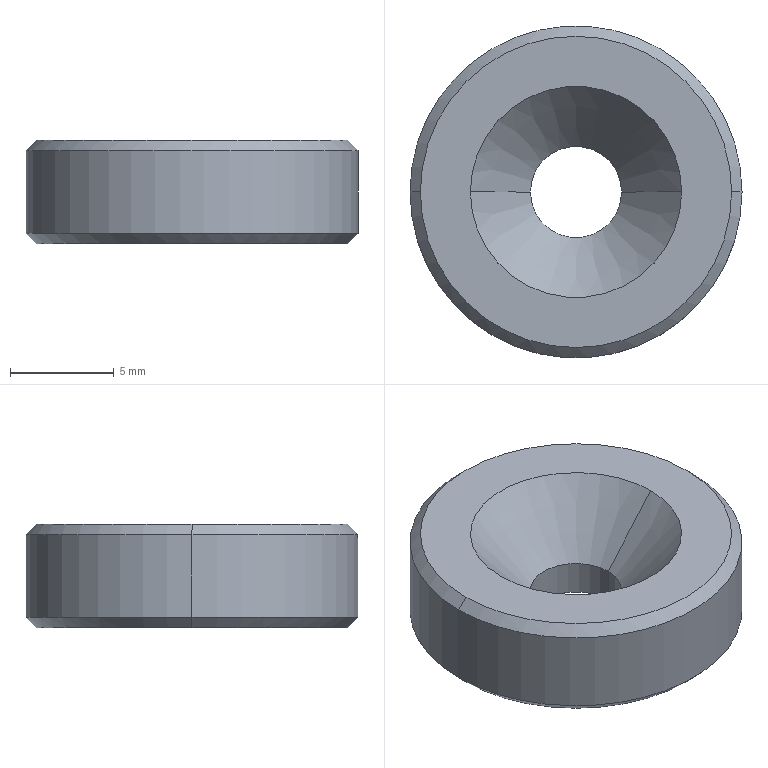Part | STEP file | 4-20.sldasm-Part-275 | 1 solid | 12 faces | box 16 x 16 x 5 mm | volume 821.609 mm3 | cone 6 | cylinder 4 | plane 2 | commonest cylinder face diameters 4.4 x2 16 x2
STEP:
#1=CARTESIAN_POINT('',(85.5,0.,-135.));
#2=VERTEX_POINT('',#1);
#3=CARTESIAN_POINT('',(100.5,0.,-135.));
#4=VERTEX_POINT('',#3);
#5=CARTESIAN_POINT('',(93.,0.,-135.));
#6=DIRECTION('',(0.,0.,1.));
#7=DIRECTION('',(-1.,0.,0.));
#8=AXIS2_PLACEMENT_3D('',#5,#6,#7);
#9=CIRCLE('',#8,7.5);
#10=EDGE_CURVE('',#2,#4,#9,.T.);
#11=ORIENTED_EDGE('',*,*,#10,.F.);
#12=CARTESIAN_POINT('',(85.,0.,-135.5));
#13=VERTEX_POINT('',#12);
#14=CARTESIAN_POINT('',(85.,0.,-135.5));
#15=DIRECTION('',(-0.7071,0.,-0.7071));
#16=VECTOR('',#15,1000.);
#17=LINE('',#14,#16);
#18=EDGE_CURVE('',#2,#13,#17,.T.);
#19=ORIENTED_EDGE('',*,*,#18,.T.);
#20=CARTESIAN_POINT('',(101.,0.,-135.5));
#21=VERTEX_POINT('',#20);
#22=CARTESIAN_POINT('',(93.,0.,-135.5));
#23=DIRECTION('',(0.,0.,-1.));
#24=DIRECTION('',(-1.,0.,0.));
#25=AXIS2_PLACEMENT_3D('',#22,#23,#24);
#26=CIRCLE('',#25,8.);
#27=EDGE_CURVE('',#21,#13,#26,.T.);
#28=ORIENTED_EDGE('',*,*,#27,.F.);
#29=CARTESIAN_POINT('',(101.,0.,-135.5));
#30=DIRECTION('',(0.7071,0.,-0.7071));
#31=VECTOR('',#30,1000.);
#32=LINE('',#29,#31);
#33=EDGE_CURVE('',#4,#21,#32,.T.);
#34=ORIENTED_EDGE('',*,*,#33,.F.);
#35=EDGE_LOOP('',(#11,#19,#28,#34));
#36=FACE_OUTER_BOUND('',#35,.T.);
#37=CARTESIAN_POINT('',(93.,0.,-135.5));
#38=DIRECTION('',(0.,0.,-1.));
#39=DIRECTION('',(1.,0.,0.));
#40=AXIS2_PLACEMENT_3D('',#37,#38,#39);
#41=CONICAL_SURFACE('',#40,8.,0.7854);
#42=ADVANCED_FACE('',(#36),#41,.T.);
#43=CARTESIAN_POINT('',(100.5,0.,-140.));
#44=VERTEX_POINT('',#43);
#45=CARTESIAN_POINT('',(85.5,0.,-140.));
#46=VERTEX_POINT('',#45);
#47=CARTESIAN_POINT('',(93.,0.,-140.));
#48=DIRECTION('',(0.,0.,-1.));
#49=DIRECTION('',(1.,0.,0.));
#50=AXIS2_PLACEMENT_3D('',#47,#48,#49);
#51=CIRCLE('',#50,7.5);
#52=EDGE_CURVE('',#44,#46,#51,.T.);
#53=ORIENTED_EDGE('',*,*,#52,.F.);
#54=CARTESIAN_POINT('',(101.,0.,-139.5));
#55=VERTEX_POINT('',#54);
#56=CARTESIAN_POINT('',(101.,0.,-139.5));
#57=DIRECTION('',(0.7071,0.,0.7071));
#58=VECTOR('',#57,1000.);
#59=LINE('',#56,#58);
#60=EDGE_CURVE('',#44,#55,#59,.T.);
#61=ORIENTED_EDGE('',*,*,#60,.T.);
#62=CARTESIAN_POINT('',(85.,0.,-139.5));
#63=VERTEX_POINT('',#62);
#64=CARTESIAN_POINT('',(93.,0.,-139.5));
#65=DIRECTION('',(0.,0.,1.));
#66=DIRECTION('',(1.,0.,0.));
#67=AXIS2_PLACEMENT_3D('',#64,#65,#66);
#68=CIRCLE('',#67,8.);
#69=EDGE_CURVE('',#63,#55,#68,.T.);
#70=ORIENTED_EDGE('',*,*,#69,.F.);
#71=CARTESIAN_POINT('',(85.,0.,-139.5));
#72=DIRECTION('',(-0.7071,0.,0.7071));
#73=VECTOR('',#72,1000.);
#74=LINE('',#71,#73);
#75=EDGE_CURVE('',#46,#63,#74,.T.);
#76=ORIENTED_EDGE('',*,*,#75,.F.);
#77=EDGE_LOOP('',(#53,#61,#70,#76));
#78=FACE_OUTER_BOUND('',#77,.T.);
#79=CARTESIAN_POINT('',(93.,0.,-139.5));
#80=DIRECTION('',(0.,0.,1.));
#81=DIRECTION('',(-1.,0.,0.));
#82=AXIS2_PLACEMENT_3D('',#79,#80,#81);
#83=CONICAL_SURFACE('',#82,8.,0.7854);
#84=ADVANCED_FACE('',(#78),#83,.T.);
#85=CARTESIAN_POINT('',(95.2,0.,-138.323));
#86=VERTEX_POINT('',#85);
#87=CARTESIAN_POINT('',(90.8,0.,-138.323));
#88=VERTEX_POINT('',#87);
#89=CARTESIAN_POINT('',(93.,0.,-138.323));
#90=DIRECTION('',(0.,0.,1.));
#91=DIRECTION('',(-1.,0.,0.));
#92=AXIS2_PLACEMENT_3D('',#89,#90,#91);
#93=CIRCLE('',#92,2.2);
#94=EDGE_CURVE('',#86,#88,#93,.T.);
#95=ORIENTED_EDGE('',*,*,#94,.F.);
#96=CARTESIAN_POINT('',(98.089,0.,-135.));
#97=VERTEX_POINT('',#96);
#98=CARTESIAN_POINT('',(98.089,0.,-135.));
#99=DIRECTION('',(0.6561,0.,0.7547));
#100=VECTOR('',#99,1000.);
#101=LINE('',#98,#100);
#102=EDGE_CURVE('',#86,#97,#101,.T.);
#103=ORIENTED_EDGE('',*,*,#102,.T.);
#104=CARTESIAN_POINT('',(87.911,0.,-135.));
#105=VERTEX_POINT('',#104);
#106=CARTESIAN_POINT('',(93.,0.,-135.));
#107=DIRECTION('',(0.,0.,1.));
#108=DIRECTION('',(-1.,0.,0.));
#109=AXIS2_PLACEMENT_3D('',#106,#107,#108);
#110=CIRCLE('',#109,5.089);
#111=EDGE_CURVE('',#97,#105,#110,.T.);
#112=ORIENTED_EDGE('',*,*,#111,.T.);
#113=CARTESIAN_POINT('',(87.911,0.,-135.));
#114=DIRECTION('',(-0.6561,0.,0.7547));
#115=VECTOR('',#114,1000.);
#116=LINE('',#113,#115);
#117=EDGE_CURVE('',#88,#105,#116,.T.);
#118=ORIENTED_EDGE('',*,*,#117,.F.);
#119=EDGE_LOOP('',(#95,#103,#112,#118));
#120=FACE_OUTER_BOUND('',#119,.T.);
#121=CARTESIAN_POINT('',(93.,0.,-135.));
#122=DIRECTION('',(0.,0.,1.));
#123=DIRECTION('',(-1.,0.,0.));
#124=AXIS2_PLACEMENT_3D('',#121,#122,#123);
#125=CONICAL_SURFACE('',#124,5.089,0.7156);
#126=ADVANCED_FACE('',(#120),#125,.F.);
#127=CARTESIAN_POINT('',(95.2,0.,-140.));
#128=VERTEX_POINT('',#127);
#129=CARTESIAN_POINT('',(90.8,0.,-140.));
#130=VERTEX_POINT('',#129);
#131=CARTESIAN_POINT('',(93.,0.,-140.));
#132=DIRECTION('',(0.,0.,1.));
#133=DIRECTION('',(-1.,0.,0.));
#134=AXIS2_PLACEMENT_3D('',#131,#132,#133);
#135=CIRCLE('',#134,2.2);
#136=EDGE_CURVE('',#128,#130,#135,.T.);
#137=ORIENTED_EDGE('',*,*,#136,.F.);
#138=CARTESIAN_POINT('',(95.2,0.,-139.));
#139=DIRECTION('',(0.,0.,1.));
#140=VECTOR('',#139,1000.);
#141=LINE('',#138,#140);
#142=EDGE_CURVE('',#128,#86,#141,.T.);
#143=ORIENTED_EDGE('',*,*,#142,.T.);
#144=ORIENTED_EDGE('',*,*,#94,.T.);
#145=CARTESIAN_POINT('',(90.8,0.,-139.));
#146=DIRECTION('',(0.,0.,1.));
#147=VECTOR('',#146,1000.);
#148=LINE('',#145,#147);
#149=EDGE_CURVE('',#130,#88,#148,.T.);
#150=ORIENTED_EDGE('',*,*,#149,.F.);
#151=EDGE_LOOP('',(#137,#143,#144,#150));
#152=FACE_OUTER_BOUND('',#151,.T.);
#153=CARTESIAN_POINT('',(93.,0.,-139.));
#154=DIRECTION('',(0.,0.,1.));
#155=DIRECTION('',(-1.,0.,0.));
#156=AXIS2_PLACEMENT_3D('',#153,#154,#155);
#157=CYLINDRICAL_SURFACE('',#156,2.2);
#158=ADVANCED_FACE('',(#152),#157,.F.);
#159=ORIENTED_EDGE('',*,*,#69,.T.);
#160=CARTESIAN_POINT('',(101.,0.,-139.));
#161=DIRECTION('',(0.,0.,1.));
#162=VECTOR('',#161,1000.);
#163=LINE('',#160,#162);
#164=EDGE_CURVE('',#55,#21,#163,.T.);
#165=ORIENTED_EDGE('',*,*,#164,.T.);
#166=ORIENTED_EDGE('',*,*,#27,.T.);
#167=CARTESIAN_POINT('',(85.,0.,-139.));
#168=DIRECTION('',(0.,0.,1.));
#169=VECTOR('',#168,1000.);
#170=LINE('',#167,#169);
#171=EDGE_CURVE('',#63,#13,#170,.T.);
#172=ORIENTED_EDGE('',*,*,#171,.F.);
#173=EDGE_LOOP('',(#159,#165,#166,#172));
#174=FACE_OUTER_BOUND('',#173,.T.);
#175=CARTESIAN_POINT('',(93.,0.,-139.));
#176=DIRECTION('',(0.,0.,1.));
#177=DIRECTION('',(-1.,0.,0.));
#178=AXIS2_PLACEMENT_3D('',#175,#176,#177);
#179=CYLINDRICAL_SURFACE('',#178,8.);
#180=ADVANCED_FACE('',(#174),#179,.T.);
#181=CARTESIAN_POINT('',(93.,0.,-135.));
#182=DIRECTION('',(0.,0.,1.));
#183=DIRECTION('',(-1.,0.,0.));
#184=AXIS2_PLACEMENT_3D('',#181,#182,#183);
#185=CIRCLE('',#184,7.5);
#186=EDGE_CURVE('',#4,#2,#185,.T.);
#187=ORIENTED_EDGE('',*,*,#186,.T.);
#188=ORIENTED_EDGE('',*,*,#10,.T.);
#189=EDGE_LOOP('',(#187,#188));
#190=FACE_OUTER_BOUND('',#189,.T.);
#191=CARTESIAN_POINT('',(93.,0.,-135.));
#192=DIRECTION('',(0.,0.,1.));
#193=DIRECTION('',(-1.,0.,0.));
#194=AXIS2_PLACEMENT_3D('',#191,#192,#193);
#195=CIRCLE('',#194,5.089);
#196=EDGE_CURVE('',#105,#97,#195,.T.);
#197=ORIENTED_EDGE('',*,*,#196,.F.);
#198=ORIENTED_EDGE('',*,*,#111,.F.);
#199=EDGE_LOOP('',(#197,#198));
#200=FACE_BOUND('',#199,.T.);
#201=CARTESIAN_POINT('',(93.,0.,-135.));
#202=DIRECTION('',(0.,0.,1.));
#203=DIRECTION('',(-1.,0.,0.));
#204=AXIS2_PLACEMENT_3D('',#201,#202,#203);
#205=PLANE('',#204);
#206=ADVANCED_FACE('',(#190,#200),#205,.T.);
#207=CARTESIAN_POINT('',(93.,0.,-140.));
#208=DIRECTION('',(0.,0.,-1.));
#209=DIRECTION('',(1.,0.,0.));
#210=AXIS2_PLACEMENT_3D('',#207,#208,#209);
#211=CIRCLE('',#210,7.5);
#212=EDGE_CURVE('',#46,#44,#211,.T.);
#213=ORIENTED_EDGE('',*,*,#212,.T.);
#214=ORIENTED_EDGE('',*,*,#52,.T.);
#215=EDGE_LOOP('',(#213,#214));
#216=FACE_OUTER_BOUND('',#215,.T.);
#217=CARTESIAN_POINT('',(93.,0.,-140.));
#218=DIRECTION('',(0.,0.,1.));
#219=DIRECTION('',(-1.,0.,0.));
#220=AXIS2_PLACEMENT_3D('',#217,#218,#219);
#221=CIRCLE('',#220,2.2);
#222=EDGE_CURVE('',#130,#128,#221,.T.);
#223=ORIENTED_EDGE('',*,*,#222,.T.);
#224=ORIENTED_EDGE('',*,*,#136,.T.);
#225=EDGE_LOOP('',(#223,#224));
#226=FACE_BOUND('',#225,.T.);
#227=CARTESIAN_POINT('',(93.,0.,-140.));
#228=DIRECTION('',(0.,0.,-1.));
#229=DIRECTION('',(1.,0.,0.));
#230=AXIS2_PLACEMENT_3D('',#227,#228,#229);
#231=PLANE('',#230);
#232=ADVANCED_FACE('',(#216,#226),#231,.T.);
#233=ORIENTED_EDGE('',*,*,#164,.F.);
#234=CARTESIAN_POINT('',(93.,0.,-139.5));
#235=DIRECTION('',(0.,0.,1.));
#236=DIRECTION('',(1.,0.,0.));
#237=AXIS2_PLACEMENT_3D('',#234,#235,#236);
#238=CIRCLE('',#237,8.);
#239=EDGE_CURVE('',#55,#63,#238,.T.);
#240=ORIENTED_EDGE('',*,*,#239,.T.);
#241=ORIENTED_EDGE('',*,*,#171,.T.);
#242=CARTESIAN_POINT('',(93.,0.,-135.5));
#243=DIRECTION('',(0.,0.,-1.));
#244=DIRECTION('',(-1.,0.,0.));
#245=AXIS2_PLACEMENT_3D('',#242,#243,#244);
#246=CIRCLE('',#245,8.);
#247=EDGE_CURVE('',#13,#21,#246,.T.);
#248=ORIENTED_EDGE('',*,*,#247,.T.);
#249=EDGE_LOOP('',(#233,#240,#241,#248));
#250=FACE_OUTER_BOUND('',#249,.T.);
#251=CARTESIAN_POINT('',(93.,0.,-139.));
#252=DIRECTION('',(0.,0.,1.));
#253=DIRECTION('',(-1.,0.,0.));
#254=AXIS2_PLACEMENT_3D('',#251,#252,#253);
#255=CYLINDRICAL_SURFACE('',#254,8.);
#256=ADVANCED_FACE('',(#250),#255,.T.);
#257=ORIENTED_EDGE('',*,*,#102,.F.);
#258=CARTESIAN_POINT('',(93.,0.,-138.323));
#259=DIRECTION('',(0.,0.,1.));
#260=DIRECTION('',(-1.,0.,0.));
#261=AXIS2_PLACEMENT_3D('',#258,#259,#260);
#262=CIRCLE('',#261,2.2);
#263=EDGE_CURVE('',#88,#86,#262,.T.);
#264=ORIENTED_EDGE('',*,*,#263,.F.);
#265=ORIENTED_EDGE('',*,*,#117,.T.);
#266=ORIENTED_EDGE('',*,*,#196,.T.);
#267=EDGE_LOOP('',(#257,#264,#265,#266));
#268=FACE_OUTER_BOUND('',#267,.T.);
#269=CARTESIAN_POINT('',(93.,0.,-135.));
#270=DIRECTION('',(0.,0.,1.));
#271=DIRECTION('',(-1.,0.,0.));
#272=AXIS2_PLACEMENT_3D('',#269,#270,#271);
#273=CONICAL_SURFACE('',#272,5.089,0.7156);
#274=ADVANCED_FACE('',(#268),#273,.F.);
#275=ORIENTED_EDGE('',*,*,#142,.F.);
#276=ORIENTED_EDGE('',*,*,#222,.F.);
#277=ORIENTED_EDGE('',*,*,#149,.T.);
#278=ORIENTED_EDGE('',*,*,#263,.T.);
#279=EDGE_LOOP('',(#275,#276,#277,#278));
#280=FACE_OUTER_BOUND('',#279,.T.);
#281=CARTESIAN_POINT('',(93.,0.,-139.));
#282=DIRECTION('',(0.,0.,1.));
#283=DIRECTION('',(-1.,0.,0.));
#284=AXIS2_PLACEMENT_3D('',#281,#282,#283);
#285=CYLINDRICAL_SURFACE('',#284,2.2);
#286=ADVANCED_FACE('',(#280),#285,.F.);
#287=ORIENTED_EDGE('',*,*,#60,.F.);
#288=ORIENTED_EDGE('',*,*,#212,.F.);
#289=ORIENTED_EDGE('',*,*,#75,.T.);
#290=ORIENTED_EDGE('',*,*,#239,.F.);
#291=EDGE_LOOP('',(#287,#288,#289,#290));
#292=FACE_OUTER_BOUND('',#291,.T.);
#293=CARTESIAN_POINT('',(93.,0.,-139.5));
#294=DIRECTION('',(0.,0.,1.));
#295=DIRECTION('',(-1.,0.,0.));
#296=AXIS2_PLACEMENT_3D('',#293,#294,#295);
#297=CONICAL_SURFACE('',#296,8.,0.7854);
#298=ADVANCED_FACE('',(#292),#297,.T.);
#299=ORIENTED_EDGE('',*,*,#18,.F.);
#300=ORIENTED_EDGE('',*,*,#186,.F.);
#301=ORIENTED_EDGE('',*,*,#33,.T.);
#302=ORIENTED_EDGE('',*,*,#247,.F.);
#303=EDGE_LOOP('',(#299,#300,#301,#302));
#304=FACE_OUTER_BOUND('',#303,.T.);
#305=CARTESIAN_POINT('',(93.,0.,-135.5));
#306=DIRECTION('',(0.,0.,-1.));
#307=DIRECTION('',(1.,0.,0.));
#308=AXIS2_PLACEMENT_3D('',#305,#306,#307);
#309=CONICAL_SURFACE('',#308,8.,0.7854);
#310=ADVANCED_FACE('',(#304),#309,.T.);
#311=CLOSED_SHELL('',(#42,#84,#126,#158,#180,#206,#232,#256,#274,#286,#298,#310));
#312=MANIFOLD_SOLID_BREP('',#311);
#313=CARTESIAN_POINT('',(0.,0.,0.));
#314=DIRECTION('',(0.,0.,1.));
#315=DIRECTION('',(1.,0.,0.));
#316=AXIS2_PLACEMENT_3D('',#313,#314,#315);
#317=(LENGTH_UNIT()NAMED_UNIT(*)SI_UNIT(.MILLI.,.METRE.));
#318=UNCERTAINTY_MEASURE_WITH_UNIT(LENGTH_MEASURE(0.00001),#317,'','');
#319=(NAMED_UNIT(*)PLANE_ANGLE_UNIT()SI_UNIT($,.RADIAN.));
#320=(NAMED_UNIT(*)SI_UNIT($,.STERADIAN.)SOLID_ANGLE_UNIT());
#321=(GEOMETRIC_REPRESENTATION_CONTEXT(3)GLOBAL_UNCERTAINTY_ASSIGNED_CONTEXT((#318))GLOBAL_UNIT_ASSIGNED_CONTEXT((#317,#319,#320))REPRESENTATION_CONTEXT('',''));
#322=ADVANCED_BREP_SHAPE_REPRESENTATION('',(#312,#316),#321);